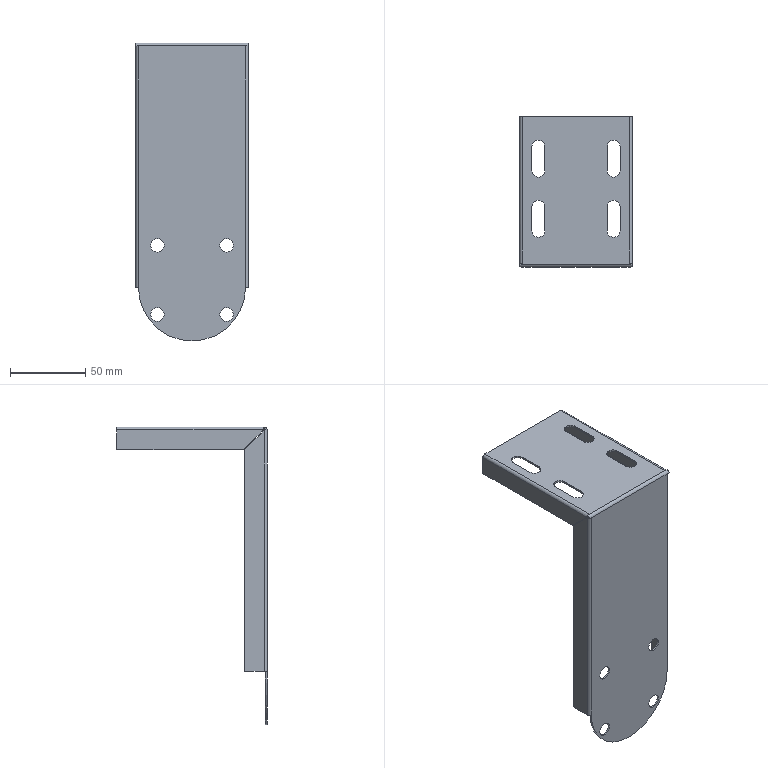Part | 1 solid | 80 faces | box 75 x 100 x 198.063 mm | volume 32396 mm3 | plane 47 | cylinder 31 | spline 2 | commonest cylinder face diameters 8.5 x12 9 x8 1.473 x5 3.873 x5 71.127 x1